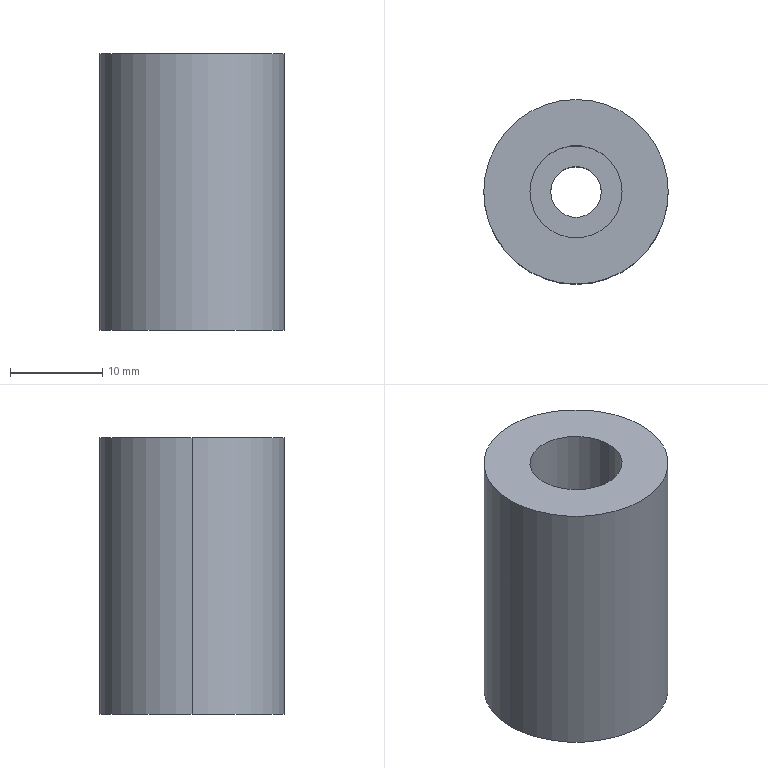Part | SolidWorks | features 3DProfileFeature 1, Extrusion 1, HoleWzd 1 | 1 solid | 9 faces | box 20 x 20 x 30 mm | volume 8055 mm3 | cylinder 6 | plane 3 | commonest cylinder face diameters 5.5 x2 10 x2 20 x2
STEP:
#1=CARTESIAN_POINT('',(-5.,0.,3.));
#2=VERTEX_POINT('',#1);
#3=CARTESIAN_POINT('',(5.,0.,3.));
#4=VERTEX_POINT('',#3);
#5=CARTESIAN_POINT('',(0.,0.,3.));
#6=DIRECTION('',(0.,0.,1.));
#7=DIRECTION('',(1.,0.,0.));
#8=AXIS2_PLACEMENT_3D('',#5,#6,#7);
#9=CIRCLE('',#8,5.);
#10=EDGE_CURVE('',#2,#4,#9,.T.);
#11=ORIENTED_EDGE('',*,*,#10,.F.);
#12=CARTESIAN_POINT('',(-5.,0.,15.));
#13=VERTEX_POINT('',#12);
#14=CARTESIAN_POINT('',(-5.,0.,15.));
#15=DIRECTION('',(0.,0.,1.));
#16=VECTOR('',#15,1000.);
#17=LINE('',#14,#16);
#18=EDGE_CURVE('',#2,#13,#17,.T.);
#19=ORIENTED_EDGE('',*,*,#18,.T.);
#20=CARTESIAN_POINT('',(5.,0.,15.));
#21=VERTEX_POINT('',#20);
#22=CARTESIAN_POINT('',(0.,0.,15.));
#23=DIRECTION('',(0.,0.,1.));
#24=DIRECTION('',(1.,0.,0.));
#25=AXIS2_PLACEMENT_3D('',#22,#23,#24);
#26=CIRCLE('',#25,5.);
#27=EDGE_CURVE('',#13,#21,#26,.T.);
#28=ORIENTED_EDGE('',*,*,#27,.T.);
#29=CARTESIAN_POINT('',(5.,0.,15.));
#30=DIRECTION('',(0.,0.,1.));
#31=VECTOR('',#30,1000.);
#32=LINE('',#29,#31);
#33=EDGE_CURVE('',#4,#21,#32,.T.);
#34=ORIENTED_EDGE('',*,*,#33,.F.);
#35=EDGE_LOOP('',(#11,#19,#28,#34));
#36=FACE_OUTER_BOUND('',#35,.T.);
#37=CARTESIAN_POINT('',(0.,0.,15.));
#38=DIRECTION('',(0.,0.,1.));
#39=DIRECTION('',(1.,0.,0.));
#40=AXIS2_PLACEMENT_3D('',#37,#38,#39);
#41=CYLINDRICAL_SURFACE('',#40,5.);
#42=ADVANCED_FACE('',(#36),#41,.F.);
#43=CARTESIAN_POINT('',(-2.75,0.,-15.));
#44=VERTEX_POINT('',#43);
#45=CARTESIAN_POINT('',(2.75,0.,-15.));
#46=VERTEX_POINT('',#45);
#47=CARTESIAN_POINT('',(0.,0.,-15.));
#48=DIRECTION('',(0.,0.,1.));
#49=DIRECTION('',(1.,0.,0.));
#50=AXIS2_PLACEMENT_3D('',#47,#48,#49);
#51=CIRCLE('',#50,2.75);
#52=EDGE_CURVE('',#44,#46,#51,.T.);
#53=ORIENTED_EDGE('',*,*,#52,.F.);
#54=CARTESIAN_POINT('',(-2.75,0.,3.));
#55=VERTEX_POINT('',#54);
#56=CARTESIAN_POINT('',(-2.75,0.,15.));
#57=DIRECTION('',(0.,0.,1.));
#58=VECTOR('',#57,1000.);
#59=LINE('',#56,#58);
#60=EDGE_CURVE('',#44,#55,#59,.T.);
#61=ORIENTED_EDGE('',*,*,#60,.T.);
#62=CARTESIAN_POINT('',(2.75,0.,3.));
#63=VERTEX_POINT('',#62);
#64=CARTESIAN_POINT('',(0.,0.,3.));
#65=DIRECTION('',(0.,0.,1.));
#66=DIRECTION('',(1.,0.,0.));
#67=AXIS2_PLACEMENT_3D('',#64,#65,#66);
#68=CIRCLE('',#67,2.75);
#69=EDGE_CURVE('',#55,#63,#68,.T.);
#70=ORIENTED_EDGE('',*,*,#69,.T.);
#71=CARTESIAN_POINT('',(2.75,0.,15.));
#72=DIRECTION('',(0.,0.,1.));
#73=VECTOR('',#72,1000.);
#74=LINE('',#71,#73);
#75=EDGE_CURVE('',#46,#63,#74,.T.);
#76=ORIENTED_EDGE('',*,*,#75,.F.);
#77=EDGE_LOOP('',(#53,#61,#70,#76));
#78=FACE_OUTER_BOUND('',#77,.T.);
#79=CARTESIAN_POINT('',(0.,0.,15.));
#80=DIRECTION('',(0.,0.,1.));
#81=DIRECTION('',(1.,0.,0.));
#82=AXIS2_PLACEMENT_3D('',#79,#80,#81);
#83=CYLINDRICAL_SURFACE('',#82,2.75);
#84=ADVANCED_FACE('',(#78),#83,.F.);
#85=CARTESIAN_POINT('',(10.,0.,15.));
#86=VERTEX_POINT('',#85);
#87=CARTESIAN_POINT('',(-10.,0.,15.));
#88=VERTEX_POINT('',#87);
#89=CARTESIAN_POINT('',(0.,0.,15.));
#90=DIRECTION('',(0.,0.,1.));
#91=DIRECTION('',(1.,0.,0.));
#92=AXIS2_PLACEMENT_3D('',#89,#90,#91);
#93=CIRCLE('',#92,10.);
#94=EDGE_CURVE('',#86,#88,#93,.T.);
#95=ORIENTED_EDGE('',*,*,#94,.F.);
#96=CARTESIAN_POINT('',(10.,0.,-15.));
#97=VERTEX_POINT('',#96);
#98=CARTESIAN_POINT('',(10.,0.,15.));
#99=DIRECTION('',(0.,0.,-1.));
#100=VECTOR('',#99,1000.);
#101=LINE('',#98,#100);
#102=EDGE_CURVE('',#86,#97,#101,.T.);
#103=ORIENTED_EDGE('',*,*,#102,.T.);
#104=CARTESIAN_POINT('',(-10.,0.,-15.));
#105=VERTEX_POINT('',#104);
#106=CARTESIAN_POINT('',(0.,0.,-15.));
#107=DIRECTION('',(0.,0.,1.));
#108=DIRECTION('',(1.,0.,0.));
#109=AXIS2_PLACEMENT_3D('',#106,#107,#108);
#110=CIRCLE('',#109,10.);
#111=EDGE_CURVE('',#97,#105,#110,.T.);
#112=ORIENTED_EDGE('',*,*,#111,.T.);
#113=CARTESIAN_POINT('',(-10.,0.,15.));
#114=DIRECTION('',(0.,0.,-1.));
#115=VECTOR('',#114,1000.);
#116=LINE('',#113,#115);
#117=EDGE_CURVE('',#88,#105,#116,.T.);
#118=ORIENTED_EDGE('',*,*,#117,.F.);
#119=EDGE_LOOP('',(#95,#103,#112,#118));
#120=FACE_OUTER_BOUND('',#119,.T.);
#121=CARTESIAN_POINT('',(0.,0.,15.));
#122=DIRECTION('',(0.,0.,-1.));
#123=DIRECTION('',(-1.,0.,0.));
#124=AXIS2_PLACEMENT_3D('',#121,#122,#123);
#125=CYLINDRICAL_SURFACE('',#124,10.);
#126=ADVANCED_FACE('',(#120),#125,.T.);
#127=ORIENTED_EDGE('',*,*,#102,.F.);
#128=CARTESIAN_POINT('',(0.,0.,15.));
#129=DIRECTION('',(0.,0.,1.));
#130=DIRECTION('',(1.,0.,0.));
#131=AXIS2_PLACEMENT_3D('',#128,#129,#130);
#132=CIRCLE('',#131,10.);
#133=EDGE_CURVE('',#88,#86,#132,.T.);
#134=ORIENTED_EDGE('',*,*,#133,.F.);
#135=ORIENTED_EDGE('',*,*,#117,.T.);
#136=CARTESIAN_POINT('',(0.,0.,-15.));
#137=DIRECTION('',(0.,0.,1.));
#138=DIRECTION('',(1.,0.,0.));
#139=AXIS2_PLACEMENT_3D('',#136,#137,#138);
#140=CIRCLE('',#139,10.);
#141=EDGE_CURVE('',#105,#97,#140,.T.);
#142=ORIENTED_EDGE('',*,*,#141,.T.);
#143=EDGE_LOOP('',(#127,#134,#135,#142));
#144=FACE_OUTER_BOUND('',#143,.T.);
#145=CARTESIAN_POINT('',(0.,0.,15.));
#146=DIRECTION('',(0.,0.,-1.));
#147=DIRECTION('',(-1.,0.,0.));
#148=AXIS2_PLACEMENT_3D('',#145,#146,#147);
#149=CYLINDRICAL_SURFACE('',#148,10.);
#150=ADVANCED_FACE('',(#144),#149,.T.);
#151=CARTESIAN_POINT('',(0.,0.,15.));
#152=DIRECTION('',(0.,0.,1.));
#153=DIRECTION('',(1.,0.,0.));
#154=AXIS2_PLACEMENT_3D('',#151,#152,#153);
#155=CIRCLE('',#154,5.);
#156=EDGE_CURVE('',#21,#13,#155,.T.);
#157=ORIENTED_EDGE('',*,*,#156,.F.);
#158=ORIENTED_EDGE('',*,*,#27,.F.);
#159=EDGE_LOOP('',(#157,#158));
#160=FACE_BOUND('',#159,.T.);
#161=ORIENTED_EDGE('',*,*,#133,.T.);
#162=ORIENTED_EDGE('',*,*,#94,.T.);
#163=EDGE_LOOP('',(#161,#162));
#164=FACE_OUTER_BOUND('',#163,.T.);
#165=CARTESIAN_POINT('',(0.,0.,15.));
#166=DIRECTION('',(0.,0.,1.));
#167=DIRECTION('',(1.,0.,0.));
#168=AXIS2_PLACEMENT_3D('',#165,#166,#167);
#169=PLANE('',#168);
#170=ADVANCED_FACE('',(#160,#164),#169,.T.);
#171=CARTESIAN_POINT('',(0.,0.,-15.));
#172=DIRECTION('',(0.,0.,1.));
#173=DIRECTION('',(1.,0.,0.));
#174=AXIS2_PLACEMENT_3D('',#171,#172,#173);
#175=CIRCLE('',#174,2.75);
#176=EDGE_CURVE('',#46,#44,#175,.T.);
#177=ORIENTED_EDGE('',*,*,#176,.T.);
#178=ORIENTED_EDGE('',*,*,#52,.T.);
#179=EDGE_LOOP('',(#177,#178));
#180=FACE_BOUND('',#179,.T.);
#181=ORIENTED_EDGE('',*,*,#141,.F.);
#182=ORIENTED_EDGE('',*,*,#111,.F.);
#183=EDGE_LOOP('',(#181,#182));
#184=FACE_OUTER_BOUND('',#183,.T.);
#185=CARTESIAN_POINT('',(0.,0.,-15.));
#186=DIRECTION('',(0.,0.,1.));
#187=DIRECTION('',(1.,0.,0.));
#188=AXIS2_PLACEMENT_3D('',#185,#186,#187);
#189=PLANE('',#188);
#190=ADVANCED_FACE('',(#180,#184),#189,.F.);
#191=ORIENTED_EDGE('',*,*,#60,.F.);
#192=ORIENTED_EDGE('',*,*,#176,.F.);
#193=ORIENTED_EDGE('',*,*,#75,.T.);
#194=CARTESIAN_POINT('',(0.,0.,3.));
#195=DIRECTION('',(0.,0.,1.));
#196=DIRECTION('',(1.,0.,0.));
#197=AXIS2_PLACEMENT_3D('',#194,#195,#196);
#198=CIRCLE('',#197,2.75);
#199=EDGE_CURVE('',#63,#55,#198,.T.);
#200=ORIENTED_EDGE('',*,*,#199,.T.);
#201=EDGE_LOOP('',(#191,#192,#193,#200));
#202=FACE_OUTER_BOUND('',#201,.T.);
#203=CARTESIAN_POINT('',(0.,0.,15.));
#204=DIRECTION('',(0.,0.,1.));
#205=DIRECTION('',(1.,0.,0.));
#206=AXIS2_PLACEMENT_3D('',#203,#204,#205);
#207=CYLINDRICAL_SURFACE('',#206,2.75);
#208=ADVANCED_FACE('',(#202),#207,.F.);
#209=ORIENTED_EDGE('',*,*,#199,.F.);
#210=ORIENTED_EDGE('',*,*,#69,.F.);
#211=EDGE_LOOP('',(#209,#210));
#212=FACE_BOUND('',#211,.T.);
#213=CARTESIAN_POINT('',(0.,0.,3.));
#214=DIRECTION('',(0.,0.,1.));
#215=DIRECTION('',(1.,0.,0.));
#216=AXIS2_PLACEMENT_3D('',#213,#214,#215);
#217=CIRCLE('',#216,5.);
#218=EDGE_CURVE('',#4,#2,#217,.T.);
#219=ORIENTED_EDGE('',*,*,#218,.T.);
#220=ORIENTED_EDGE('',*,*,#10,.T.);
#221=EDGE_LOOP('',(#219,#220));
#222=FACE_OUTER_BOUND('',#221,.T.);
#223=CARTESIAN_POINT('',(2.75,0.,3.));
#224=DIRECTION('',(0.,0.,-1.));
#225=DIRECTION('',(-1.,0.,0.));
#226=AXIS2_PLACEMENT_3D('',#223,#224,#225);
#227=PLANE('',#226);
#228=ADVANCED_FACE('',(#212,#222),#227,.F.);
#229=ORIENTED_EDGE('',*,*,#18,.F.);
#230=ORIENTED_EDGE('',*,*,#218,.F.);
#231=ORIENTED_EDGE('',*,*,#33,.T.);
#232=ORIENTED_EDGE('',*,*,#156,.T.);
#233=EDGE_LOOP('',(#229,#230,#231,#232));
#234=FACE_OUTER_BOUND('',#233,.T.);
#235=CARTESIAN_POINT('',(0.,0.,15.));
#236=DIRECTION('',(0.,0.,1.));
#237=DIRECTION('',(1.,0.,0.));
#238=AXIS2_PLACEMENT_3D('',#235,#236,#237);
#239=CYLINDRICAL_SURFACE('',#238,5.);
#240=ADVANCED_FACE('',(#234),#239,.F.);
#241=CLOSED_SHELL('',(#42,#84,#126,#150,#170,#190,#208,#228,#240));
#242=MANIFOLD_SOLID_BREP('',#241);
#243=CARTESIAN_POINT('',(0.,0.,0.));
#244=DIRECTION('',(0.,0.,1.));
#245=DIRECTION('',(1.,0.,0.));
#246=AXIS2_PLACEMENT_3D('',#243,#244,#245);
#247=(LENGTH_UNIT()NAMED_UNIT(*)SI_UNIT(.MILLI.,.METRE.));
#248=UNCERTAINTY_MEASURE_WITH_UNIT(LENGTH_MEASURE(0.00001),#247,'','');
#249=(NAMED_UNIT(*)PLANE_ANGLE_UNIT()SI_UNIT($,.RADIAN.));
#250=(NAMED_UNIT(*)SI_UNIT($,.STERADIAN.)SOLID_ANGLE_UNIT());
#251=(GEOMETRIC_REPRESENTATION_CONTEXT(3)GLOBAL_UNCERTAINTY_ASSIGNED_CONTEXT((#248))GLOBAL_UNIT_ASSIGNED_CONTEXT((#247,#249,#250))REPRESENTATION_CONTEXT('',''));
#252=ADVANCED_BREP_SHAPE_REPRESENTATION('',(#242,#246),#251);